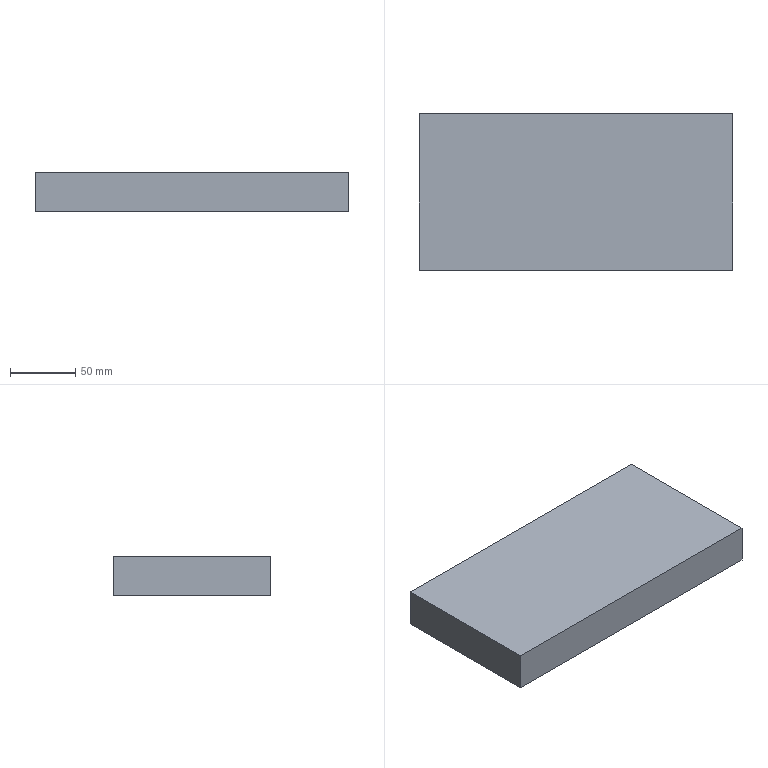Part | SolidWorks | features Extrusion 1 | 1 solid | 6 faces | box 240 x 120 x 30 mm | volume 864000 mm3 | plane 6
STEP:
#1=CARTESIAN_POINT('',(-31.657,99.343,0.));
#2=VERTEX_POINT('',#1);
#3=CARTESIAN_POINT('',(-31.657,-20.657,0.));
#4=VERTEX_POINT('',#3);
#5=CARTESIAN_POINT('',(-31.657,99.343,0.));
#6=DIRECTION('',(0.,-1.,0.));
#7=VECTOR('',#6,1000.);
#8=LINE('',#5,#7);
#9=EDGE_CURVE('',#2,#4,#8,.T.);
#10=ORIENTED_EDGE('',*,*,#9,.T.);
#11=CARTESIAN_POINT('',(-31.657,-20.657,30.));
#12=VERTEX_POINT('',#11);
#13=CARTESIAN_POINT('',(-31.657,-20.657,30.));
#14=DIRECTION('',(0.,0.,-1.));
#15=VECTOR('',#14,1000.);
#16=LINE('',#13,#15);
#17=EDGE_CURVE('',#12,#4,#16,.T.);
#18=ORIENTED_EDGE('',*,*,#17,.F.);
#19=CARTESIAN_POINT('',(-31.657,99.343,30.));
#20=VERTEX_POINT('',#19);
#21=CARTESIAN_POINT('',(-31.657,99.343,30.));
#22=DIRECTION('',(0.,-1.,0.));
#23=VECTOR('',#22,1000.);
#24=LINE('',#21,#23);
#25=EDGE_CURVE('',#20,#12,#24,.T.);
#26=ORIENTED_EDGE('',*,*,#25,.F.);
#27=CARTESIAN_POINT('',(-31.657,99.343,30.));
#28=DIRECTION('',(0.,0.,-1.));
#29=VECTOR('',#28,1000.);
#30=LINE('',#27,#29);
#31=EDGE_CURVE('',#20,#2,#30,.T.);
#32=ORIENTED_EDGE('',*,*,#31,.T.);
#33=EDGE_LOOP('',(#10,#18,#26,#32));
#34=FACE_OUTER_BOUND('',#33,.T.);
#35=CARTESIAN_POINT('',(-31.657,99.343,30.));
#36=DIRECTION('',(1.,0.,0.));
#37=DIRECTION('',(0.,1.,0.));
#38=AXIS2_PLACEMENT_3D('',#35,#36,#37);
#39=PLANE('',#38);
#40=ADVANCED_FACE('',(#34),#39,.F.);
#41=CARTESIAN_POINT('',(208.343,-20.657,0.));
#42=VERTEX_POINT('',#41);
#43=CARTESIAN_POINT('',(-31.657,-20.657,0.));
#44=DIRECTION('',(1.,0.,0.));
#45=VECTOR('',#44,1000.);
#46=LINE('',#43,#45);
#47=EDGE_CURVE('',#4,#42,#46,.T.);
#48=ORIENTED_EDGE('',*,*,#47,.T.);
#49=CARTESIAN_POINT('',(208.343,-20.657,30.));
#50=VERTEX_POINT('',#49);
#51=CARTESIAN_POINT('',(208.343,-20.657,30.));
#52=DIRECTION('',(0.,0.,-1.));
#53=VECTOR('',#52,1000.);
#54=LINE('',#51,#53);
#55=EDGE_CURVE('',#50,#42,#54,.T.);
#56=ORIENTED_EDGE('',*,*,#55,.F.);
#57=CARTESIAN_POINT('',(-31.657,-20.657,30.));
#58=DIRECTION('',(1.,0.,0.));
#59=VECTOR('',#58,1000.);
#60=LINE('',#57,#59);
#61=EDGE_CURVE('',#12,#50,#60,.T.);
#62=ORIENTED_EDGE('',*,*,#61,.F.);
#63=ORIENTED_EDGE('',*,*,#17,.T.);
#64=EDGE_LOOP('',(#48,#56,#62,#63));
#65=FACE_OUTER_BOUND('',#64,.T.);
#66=CARTESIAN_POINT('',(-31.657,-20.657,30.));
#67=DIRECTION('',(0.,1.,0.));
#68=DIRECTION('',(0.,0.,1.));
#69=AXIS2_PLACEMENT_3D('',#66,#67,#68);
#70=PLANE('',#69);
#71=ADVANCED_FACE('',(#65),#70,.F.);
#72=CARTESIAN_POINT('',(208.343,99.343,0.));
#73=VERTEX_POINT('',#72);
#74=CARTESIAN_POINT('',(208.343,99.343,0.));
#75=DIRECTION('',(0.,1.,0.));
#76=VECTOR('',#75,1000.);
#77=LINE('',#74,#76);
#78=EDGE_CURVE('',#42,#73,#77,.T.);
#79=ORIENTED_EDGE('',*,*,#78,.T.);
#80=CARTESIAN_POINT('',(208.343,99.343,30.));
#81=VERTEX_POINT('',#80);
#82=CARTESIAN_POINT('',(208.343,99.343,30.));
#83=DIRECTION('',(0.,0.,-1.));
#84=VECTOR('',#83,1000.);
#85=LINE('',#82,#84);
#86=EDGE_CURVE('',#81,#73,#85,.T.);
#87=ORIENTED_EDGE('',*,*,#86,.F.);
#88=CARTESIAN_POINT('',(208.343,99.343,30.));
#89=DIRECTION('',(0.,1.,0.));
#90=VECTOR('',#89,1000.);
#91=LINE('',#88,#90);
#92=EDGE_CURVE('',#50,#81,#91,.T.);
#93=ORIENTED_EDGE('',*,*,#92,.F.);
#94=ORIENTED_EDGE('',*,*,#55,.T.);
#95=EDGE_LOOP('',(#79,#87,#93,#94));
#96=FACE_OUTER_BOUND('',#95,.T.);
#97=CARTESIAN_POINT('',(208.343,99.343,30.));
#98=DIRECTION('',(-1.,0.,0.));
#99=DIRECTION('',(0.,-1.,0.));
#100=AXIS2_PLACEMENT_3D('',#97,#98,#99);
#101=PLANE('',#100);
#102=ADVANCED_FACE('',(#96),#101,.F.);
#103=CARTESIAN_POINT('',(-31.657,99.343,0.));
#104=DIRECTION('',(-1.,0.,0.));
#105=VECTOR('',#104,1000.);
#106=LINE('',#103,#105);
#107=EDGE_CURVE('',#73,#2,#106,.T.);
#108=ORIENTED_EDGE('',*,*,#107,.T.);
#109=ORIENTED_EDGE('',*,*,#31,.F.);
#110=CARTESIAN_POINT('',(-31.657,99.343,30.));
#111=DIRECTION('',(-1.,0.,0.));
#112=VECTOR('',#111,1000.);
#113=LINE('',#110,#112);
#114=EDGE_CURVE('',#81,#20,#113,.T.);
#115=ORIENTED_EDGE('',*,*,#114,.F.);
#116=ORIENTED_EDGE('',*,*,#86,.T.);
#117=EDGE_LOOP('',(#108,#109,#115,#116));
#118=FACE_OUTER_BOUND('',#117,.T.);
#119=CARTESIAN_POINT('',(-31.657,99.343,30.));
#120=DIRECTION('',(0.,-1.,0.));
#121=DIRECTION('',(0.,0.,-1.));
#122=AXIS2_PLACEMENT_3D('',#119,#120,#121);
#123=PLANE('',#122);
#124=ADVANCED_FACE('',(#118),#123,.F.);
#125=ORIENTED_EDGE('',*,*,#25,.T.);
#126=ORIENTED_EDGE('',*,*,#61,.T.);
#127=ORIENTED_EDGE('',*,*,#92,.T.);
#128=ORIENTED_EDGE('',*,*,#114,.T.);
#129=EDGE_LOOP('',(#125,#126,#127,#128));
#130=FACE_OUTER_BOUND('',#129,.T.);
#131=CARTESIAN_POINT('',(0.,0.,30.));
#132=DIRECTION('',(0.,0.,1.));
#133=DIRECTION('',(1.,0.,0.));
#134=AXIS2_PLACEMENT_3D('',#131,#132,#133);
#135=PLANE('',#134);
#136=ADVANCED_FACE('',(#130),#135,.T.);
#137=ORIENTED_EDGE('',*,*,#9,.F.);
#138=ORIENTED_EDGE('',*,*,#107,.F.);
#139=ORIENTED_EDGE('',*,*,#78,.F.);
#140=ORIENTED_EDGE('',*,*,#47,.F.);
#141=EDGE_LOOP('',(#137,#138,#139,#140));
#142=FACE_OUTER_BOUND('',#141,.T.);
#143=CARTESIAN_POINT('',(0.,0.,0.));
#144=DIRECTION('',(0.,0.,1.));
#145=DIRECTION('',(1.,0.,0.));
#146=AXIS2_PLACEMENT_3D('',#143,#144,#145);
#147=PLANE('',#146);
#148=ADVANCED_FACE('',(#142),#147,.F.);
#149=CLOSED_SHELL('',(#40,#71,#102,#124,#136,#148));
#150=MANIFOLD_SOLID_BREP('',#149);
#151=CARTESIAN_POINT('',(0.,0.,0.));
#152=DIRECTION('',(0.,0.,1.));
#153=DIRECTION('',(1.,0.,0.));
#154=AXIS2_PLACEMENT_3D('',#151,#152,#153);
#155=(LENGTH_UNIT()NAMED_UNIT(*)SI_UNIT(.MILLI.,.METRE.));
#156=UNCERTAINTY_MEASURE_WITH_UNIT(LENGTH_MEASURE(0.00001),#155,'','');
#157=(NAMED_UNIT(*)PLANE_ANGLE_UNIT()SI_UNIT($,.RADIAN.));
#158=(NAMED_UNIT(*)SI_UNIT($,.STERADIAN.)SOLID_ANGLE_UNIT());
#159=(GEOMETRIC_REPRESENTATION_CONTEXT(3)GLOBAL_UNCERTAINTY_ASSIGNED_CONTEXT((#156))GLOBAL_UNIT_ASSIGNED_CONTEXT((#155,#157,#158))REPRESENTATION_CONTEXT('',''));
#160=ADVANCED_BREP_SHAPE_REPRESENTATION('',(#150,#154),#159);